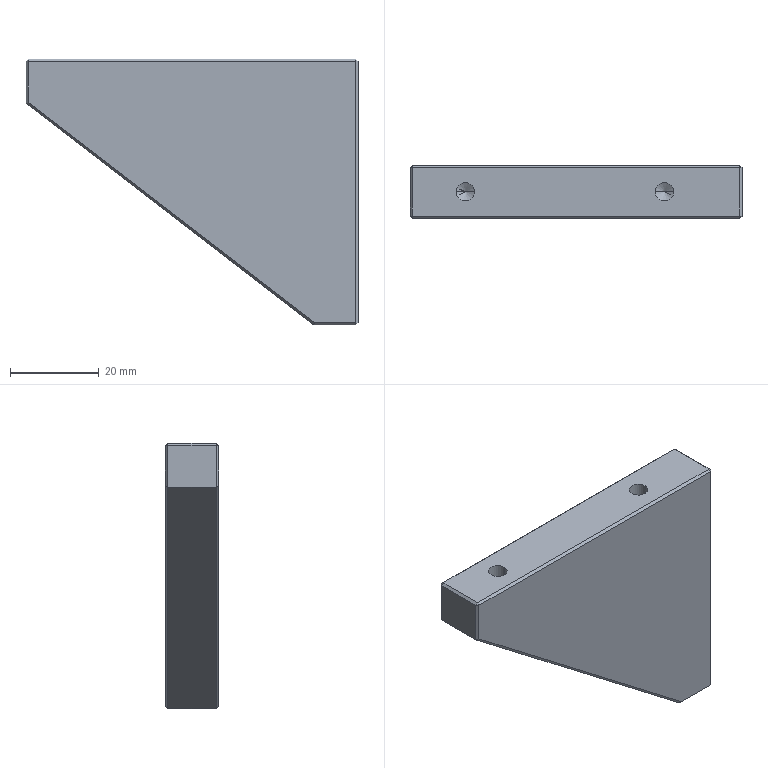Part | STEP file | ND25021-01-JDKM-62-TL | 1 solid | 42 faces | box 75 x 12 x 60 mm | volume 33726 mm3 | plane 26 | cylinder 8 | cone 8 | commonest cylinder face diameters 4.2 x8